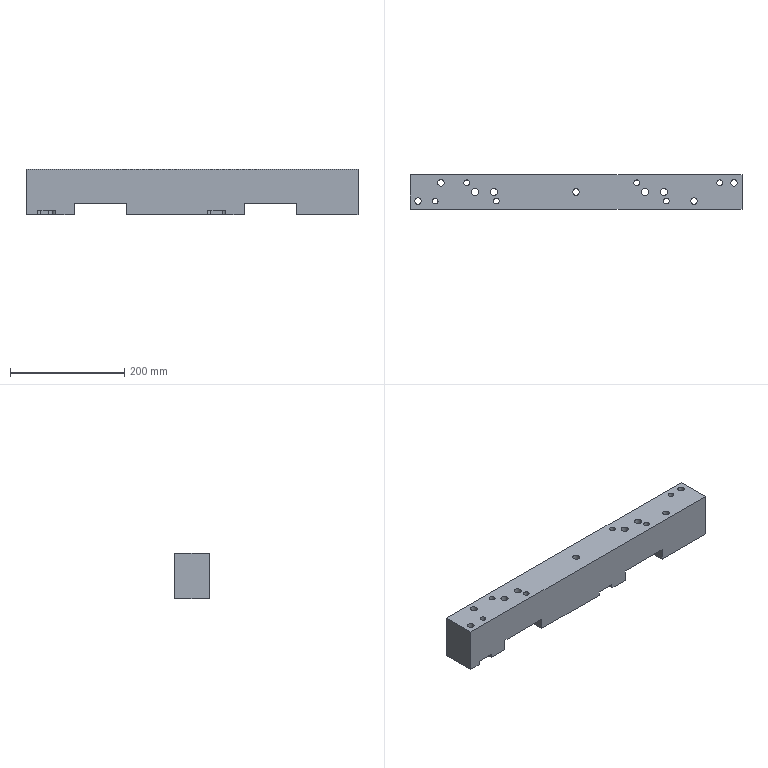Part | STEP file | lll_id3490_x_t | 1 solid | 78 faces | box 580 x 60 x 80 mm | volume 2402924 mm3 | plane 37 | cylinder 35 | cone 6 | commonest cylinder face diameters 10 x12 8.505 x6 12.5 x6 18.007 x6 11.509 x5